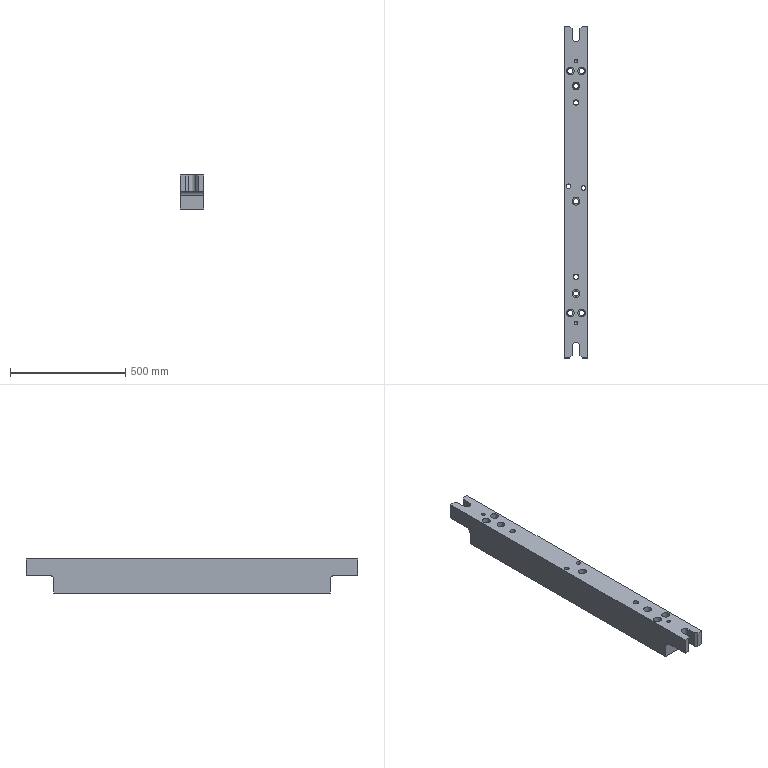Part | STEP file | lll_id2302_x_t | 1 solid | 57 faces | box 100 x 1440 x 147.5 mm | volume 18089858 mm3 | plane 29 | cylinder 26 | cone 2 | commonest cylinder face diameters 23.009 x7 34.008 x7 20 x4 14.506 x2 24 x2 34 x2
STEP:
#1=CARTESIAN_POINT('',(345.5,24.75,222.5));
#2=VERTEX_POINT('',#1);
#3=CARTESIAN_POINT('',(335.5,24.75,222.5));
#4=DIRECTION('',(0.,0.,1.));
#5=DIRECTION('',(1.,0.,0.));
#6=AXIS2_PLACEMENT_3D('',#3,#4,#5);
#7=CIRCLE('',#6,10.);
#8=EDGE_CURVE('',#2,#2,#7,.T.);
#9=ORIENTED_EDGE('',*,*,#8,.T.);
#10=EDGE_LOOP('',(#9));
#11=FACE_BOUND('',#10,.T.);
#12=CARTESIAN_POINT('',(317.435,-600.,222.5));
#13=VERTEX_POINT('',#12);
#14=CARTESIAN_POINT('',(317.435,600.,222.5));
#15=VERTEX_POINT('',#14);
#16=CARTESIAN_POINT('',(317.435,-1.,222.5));
#17=DIRECTION('',(0.,1.,0.));
#18=VECTOR('',#17,1.);
#19=LINE('',#16,#18);
#20=EDGE_CURVE('',#13,#15,#19,.T.);
#21=ORIENTED_EDGE('',*,*,#20,.T.);
#22=CARTESIAN_POINT('',(417.435,600.,222.5));
#23=VERTEX_POINT('',#22);
#24=CARTESIAN_POINT('',(-1848.88,600.,222.5));
#25=DIRECTION('',(1.,0.,0.));
#26=VECTOR('',#25,1.);
#27=LINE('',#24,#26);
#28=EDGE_CURVE('',#15,#23,#27,.T.);
#29=ORIENTED_EDGE('',*,*,#28,.T.);
#30=CARTESIAN_POINT('',(417.435,-600.,222.5));
#31=VERTEX_POINT('',#30);
#32=CARTESIAN_POINT('',(417.435,-1.,222.5));
#33=DIRECTION('',(0.,1.,0.));
#34=VECTOR('',#33,1.);
#35=LINE('',#32,#34);
#36=EDGE_CURVE('',#31,#23,#35,.T.);
#37=ORIENTED_EDGE('',*,*,#36,.F.);
#38=CARTESIAN_POINT('',(-1848.88,-600.,222.5));
#39=DIRECTION('',(-1.,0.,0.));
#40=VECTOR('',#39,1.);
#41=LINE('',#38,#40);
#42=EDGE_CURVE('',#31,#13,#41,.T.);
#43=ORIENTED_EDGE('',*,*,#42,.T.);
#44=EDGE_LOOP('',(#21,#29,#37,#43));
#45=FACE_BOUND('',#44,.T.);
#46=CARTESIAN_POINT('',(380.931,-525.,222.5));
#47=VERTEX_POINT('',#46);
#48=CARTESIAN_POINT('',(392.435,-525.,222.5));
#49=DIRECTION('',(0.,0.,-1.));
#50=DIRECTION('',(-1.,0.,0.));
#51=AXIS2_PLACEMENT_3D('',#48,#49,#50);
#52=CIRCLE('',#51,11.505);
#53=EDGE_CURVE('',#47,#47,#52,.T.);
#54=ORIENTED_EDGE('',*,*,#53,.F.);
#55=EDGE_LOOP('',(#54));
#56=FACE_BOUND('',#55,.T.);
#57=CARTESIAN_POINT('',(357.435,-368.,222.5));
#58=VERTEX_POINT('',#57);
#59=CARTESIAN_POINT('',(367.435,-368.,222.5));
#60=DIRECTION('',(0.,0.,-1.));
#61=DIRECTION('',(-1.,0.,0.));
#62=AXIS2_PLACEMENT_3D('',#59,#60,#61);
#63=CIRCLE('',#62,10.);
#64=EDGE_CURVE('',#58,#58,#63,.T.);
#65=ORIENTED_EDGE('',*,*,#64,.F.);
#66=EDGE_LOOP('',(#65));
#67=FACE_BOUND('',#66,.T.);
#68=CARTESIAN_POINT('',(355.931,-440.,222.5));
#69=VERTEX_POINT('',#68);
#70=CARTESIAN_POINT('',(367.435,-440.,222.5));
#71=DIRECTION('',(0.,0.,-1.));
#72=DIRECTION('',(-1.,0.,0.));
#73=AXIS2_PLACEMENT_3D('',#70,#71,#72);
#74=CIRCLE('',#73,11.505);
#75=EDGE_CURVE('',#69,#69,#74,.T.);
#76=ORIENTED_EDGE('',*,*,#75,.F.);
#77=EDGE_LOOP('',(#76));
#78=FACE_BOUND('',#77,.T.);
#79=CARTESIAN_POINT('',(330.931,-525.,222.5));
#80=VERTEX_POINT('',#79);
#81=CARTESIAN_POINT('',(342.435,-525.,222.5));
#82=DIRECTION('',(0.,0.,-1.));
#83=DIRECTION('',(-1.,0.,0.));
#84=AXIS2_PLACEMENT_3D('',#81,#82,#83);
#85=CIRCLE('',#84,11.505);
#86=EDGE_CURVE('',#80,#80,#85,.T.);
#87=ORIENTED_EDGE('',*,*,#86,.F.);
#88=EDGE_LOOP('',(#87));
#89=FACE_BOUND('',#88,.T.);
#90=CARTESIAN_POINT('',(353.94,525.,222.5));
#91=VERTEX_POINT('',#90);
#92=CARTESIAN_POINT('',(342.435,525.,222.5));
#93=DIRECTION('',(0.,0.,-1.));
#94=DIRECTION('',(1.,0.,0.));
#95=AXIS2_PLACEMENT_3D('',#92,#93,#94);
#96=CIRCLE('',#95,11.505);
#97=EDGE_CURVE('',#91,#91,#96,.T.);
#98=ORIENTED_EDGE('',*,*,#97,.F.);
#99=EDGE_LOOP('',(#98));
#100=FACE_BOUND('',#99,.T.);
#101=CARTESIAN_POINT('',(403.94,525.,222.5));
#102=VERTEX_POINT('',#101);
#103=CARTESIAN_POINT('',(392.435,525.,222.5));
#104=DIRECTION('',(0.,0.,-1.));
#105=DIRECTION('',(1.,0.,0.));
#106=AXIS2_PLACEMENT_3D('',#103,#104,#105);
#107=CIRCLE('',#106,11.505);
#108=EDGE_CURVE('',#102,#102,#107,.T.);
#109=ORIENTED_EDGE('',*,*,#108,.F.);
#110=EDGE_LOOP('',(#109));
#111=FACE_BOUND('',#110,.T.);
#112=CARTESIAN_POINT('',(378.94,460.,222.5));
#113=VERTEX_POINT('',#112);
#114=CARTESIAN_POINT('',(367.435,460.,222.5));
#115=DIRECTION('',(0.,0.,-1.));
#116=DIRECTION('',(1.,0.,0.));
#117=AXIS2_PLACEMENT_3D('',#114,#115,#116);
#118=CIRCLE('',#117,11.505);
#119=EDGE_CURVE('',#113,#113,#118,.T.);
#120=ORIENTED_EDGE('',*,*,#119,.F.);
#121=EDGE_LOOP('',(#120));
#122=FACE_BOUND('',#121,.T.);
#123=CARTESIAN_POINT('',(378.94,-40.,222.5));
#124=VERTEX_POINT('',#123);
#125=CARTESIAN_POINT('',(367.435,-40.,222.5));
#126=DIRECTION('',(0.,0.,-1.));
#127=DIRECTION('',(1.,0.,0.));
#128=AXIS2_PLACEMENT_3D('',#125,#126,#127);
#129=CIRCLE('',#128,11.505);
#130=EDGE_CURVE('',#124,#124,#129,.T.);
#131=ORIENTED_EDGE('',*,*,#130,.F.);
#132=EDGE_LOOP('',(#131));
#133=FACE_BOUND('',#132,.T.);
#134=CARTESIAN_POINT('',(377.435,388.,222.5));
#135=VERTEX_POINT('',#134);
#136=CARTESIAN_POINT('',(367.435,388.,222.5));
#137=DIRECTION('',(0.,0.,1.));
#138=DIRECTION('',(1.,0.,0.));
#139=AXIS2_PLACEMENT_3D('',#136,#137,#138);
#140=CIRCLE('',#139,10.);
#141=EDGE_CURVE('',#135,#135,#140,.T.);
#142=ORIENTED_EDGE('',*,*,#141,.T.);
#143=EDGE_LOOP('',(#142));
#144=FACE_BOUND('',#143,.T.);
#145=CARTESIAN_POINT('',(410.5,17.75,222.5));
#146=VERTEX_POINT('',#145);
#147=CARTESIAN_POINT('',(400.5,17.75,222.5));
#148=DIRECTION('',(0.,0.,1.));
#149=DIRECTION('',(1.,0.,0.));
#150=AXIS2_PLACEMENT_3D('',#147,#148,#149);
#151=CIRCLE('',#150,10.);
#152=EDGE_CURVE('',#146,#146,#151,.T.);
#153=ORIENTED_EDGE('',*,*,#152,.T.);
#154=EDGE_LOOP('',(#153));
#155=FACE_BOUND('',#154,.T.);
#156=CARTESIAN_POINT('',(-1848.88,-1.,222.5));
#157=DIRECTION('',(0.,0.,-1.));
#158=DIRECTION('',(1.,0.,0.));
#159=AXIS2_PLACEMENT_3D('',#156,#157,#158);
#160=PLANE('',#159);
#161=ADVANCED_FACE('',(#11,#45,#56,#67,#78,#89,#100,#111,#122,#133,#144,#155),#160,.T.);
#162=CARTESIAN_POINT('',(390.5,17.75,370.));
#163=VERTEX_POINT('',#162);
#164=CARTESIAN_POINT('',(400.5,17.75,370.));
#165=DIRECTION('',(0.,0.,-1.));
#166=DIRECTION('',(-1.,0.,0.));
#167=AXIS2_PLACEMENT_3D('',#164,#165,#166);
#168=CIRCLE('',#167,10.);
#169=EDGE_CURVE('',#163,#163,#168,.T.);
#170=ORIENTED_EDGE('',*,*,#169,.T.);
#171=EDGE_LOOP('',(#170));
#172=FACE_BOUND('',#171,.T.);
#173=CARTESIAN_POINT('',(325.5,24.75,370.));
#174=VERTEX_POINT('',#173);
#175=CARTESIAN_POINT('',(335.5,24.75,370.));
#176=DIRECTION('',(0.,0.,-1.));
#177=DIRECTION('',(-1.,0.,0.));
#178=AXIS2_PLACEMENT_3D('',#175,#176,#177);
#179=CIRCLE('',#178,10.);
#180=EDGE_CURVE('',#174,#174,#179,.T.);
#181=ORIENTED_EDGE('',*,*,#180,.T.);
#182=EDGE_LOOP('',(#181));
#183=FACE_BOUND('',#182,.T.);
#184=CARTESIAN_POINT('',(317.435,-720.,370.));
#185=VERTEX_POINT('',#184);
#186=CARTESIAN_POINT('',(317.435,720.,370.));
#187=VERTEX_POINT('',#186);
#188=CARTESIAN_POINT('',(317.435,-1.,370.));
#189=DIRECTION('',(0.,1.,0.));
#190=VECTOR('',#189,1.);
#191=LINE('',#188,#190);
#192=EDGE_CURVE('',#185,#187,#191,.T.);
#193=ORIENTED_EDGE('',*,*,#192,.F.);
#194=CARTESIAN_POINT('',(340.435,-720.,370.));
#195=VERTEX_POINT('',#194);
#196=CARTESIAN_POINT('',(-1848.88,-720.,370.));
#197=DIRECTION('',(-1.,0.,0.));
#198=VECTOR('',#197,1.);
#199=LINE('',#196,#198);
#200=EDGE_CURVE('',#195,#185,#199,.T.);
#201=ORIENTED_EDGE('',*,*,#200,.F.);
#202=CARTESIAN_POINT('',(350.435,-710.,370.));
#203=VERTEX_POINT('',#202);
#204=CARTESIAN_POINT('',(350.435,-710.,370.));
#205=DIRECTION('',(0.7071,0.7071,0.));
#206=VECTOR('',#205,1.);
#207=LINE('',#204,#206);
#208=EDGE_CURVE('',#195,#203,#207,.T.);
#209=ORIENTED_EDGE('',*,*,#208,.T.);
#210=CARTESIAN_POINT('',(350.435,-670.,370.));
#211=VERTEX_POINT('',#210);
#212=CARTESIAN_POINT('',(350.435,120.,370.));
#213=DIRECTION('',(0.,-1.,0.));
#214=VECTOR('',#213,1.);
#215=LINE('',#212,#214);
#216=EDGE_CURVE('',#211,#203,#215,.T.);
#217=ORIENTED_EDGE('',*,*,#216,.F.);
#218=CARTESIAN_POINT('',(384.435,-670.,370.));
#219=VERTEX_POINT('',#218);
#220=CARTESIAN_POINT('',(367.435,-670.,370.));
#221=DIRECTION('',(0.,0.,1.));
#222=DIRECTION('',(1.,0.,0.));
#223=AXIS2_PLACEMENT_3D('',#220,#221,#222);
#224=CIRCLE('',#223,17.);
#225=EDGE_CURVE('',#219,#211,#224,.T.);
#226=ORIENTED_EDGE('',*,*,#225,.F.);
#227=CARTESIAN_POINT('',(384.435,-710.,370.));
#228=VERTEX_POINT('',#227);
#229=CARTESIAN_POINT('',(384.435,120.,370.));
#230=DIRECTION('',(0.,1.,0.));
#231=VECTOR('',#230,1.);
#232=LINE('',#229,#231);
#233=EDGE_CURVE('',#228,#219,#232,.T.);
#234=ORIENTED_EDGE('',*,*,#233,.F.);
#235=CARTESIAN_POINT('',(394.435,-720.,370.));
#236=VERTEX_POINT('',#235);
#237=CARTESIAN_POINT('',(384.435,-710.,370.));
#238=DIRECTION('',(0.7071,-0.7071,0.));
#239=VECTOR('',#238,1.);
#240=LINE('',#237,#239);
#241=EDGE_CURVE('',#228,#236,#240,.T.);
#242=ORIENTED_EDGE('',*,*,#241,.T.);
#243=CARTESIAN_POINT('',(417.435,-720.,370.));
#244=VERTEX_POINT('',#243);
#245=CARTESIAN_POINT('',(-1848.88,-720.,370.));
#246=DIRECTION('',(-1.,0.,0.));
#247=VECTOR('',#246,1.);
#248=LINE('',#245,#247);
#249=EDGE_CURVE('',#244,#236,#248,.T.);
#250=ORIENTED_EDGE('',*,*,#249,.F.);
#251=CARTESIAN_POINT('',(417.435,720.,370.));
#252=VERTEX_POINT('',#251);
#253=CARTESIAN_POINT('',(417.435,0.,370.));
#254=DIRECTION('',(0.,-1.,0.));
#255=VECTOR('',#254,1.);
#256=LINE('',#253,#255);
#257=EDGE_CURVE('',#252,#244,#256,.T.);
#258=ORIENTED_EDGE('',*,*,#257,.F.);
#259=CARTESIAN_POINT('',(394.435,720.,370.));
#260=VERTEX_POINT('',#259);
#261=CARTESIAN_POINT('',(-1848.88,720.,370.));
#262=DIRECTION('',(1.,0.,0.));
#263=VECTOR('',#262,1.);
#264=LINE('',#261,#263);
#265=EDGE_CURVE('',#260,#252,#264,.T.);
#266=ORIENTED_EDGE('',*,*,#265,.F.);
#267=CARTESIAN_POINT('',(384.435,710.,370.));
#268=VERTEX_POINT('',#267);
#269=CARTESIAN_POINT('',(350.935,676.5,370.));
#270=DIRECTION('',(0.7071,0.7071,0.));
#271=VECTOR('',#270,1.);
#272=LINE('',#269,#271);
#273=EDGE_CURVE('',#268,#260,#272,.T.);
#274=ORIENTED_EDGE('',*,*,#273,.F.);
#275=CARTESIAN_POINT('',(384.435,670.,370.));
#276=VERTEX_POINT('',#275);
#277=CARTESIAN_POINT('',(384.435,-120.,370.));
#278=DIRECTION('',(0.,-1.,0.));
#279=VECTOR('',#278,1.);
#280=LINE('',#277,#279);
#281=EDGE_CURVE('',#268,#276,#280,.T.);
#282=ORIENTED_EDGE('',*,*,#281,.T.);
#283=CARTESIAN_POINT('',(350.435,670.,370.));
#284=VERTEX_POINT('',#283);
#285=CARTESIAN_POINT('',(367.435,670.,370.));
#286=DIRECTION('',(0.,0.,-1.));
#287=DIRECTION('',(1.,0.,0.));
#288=AXIS2_PLACEMENT_3D('',#285,#286,#287);
#289=CIRCLE('',#288,17.);
#290=EDGE_CURVE('',#276,#284,#289,.T.);
#291=ORIENTED_EDGE('',*,*,#290,.T.);
#292=CARTESIAN_POINT('',(350.435,710.,370.));
#293=VERTEX_POINT('',#292);
#294=CARTESIAN_POINT('',(350.435,-120.,370.));
#295=DIRECTION('',(0.,1.,0.));
#296=VECTOR('',#295,1.);
#297=LINE('',#294,#296);
#298=EDGE_CURVE('',#284,#293,#297,.T.);
#299=ORIENTED_EDGE('',*,*,#298,.T.);
#300=CARTESIAN_POINT('',(340.435,720.,370.));
#301=VERTEX_POINT('',#300);
#302=CARTESIAN_POINT('',(1043.935,16.5,370.));
#303=DIRECTION('',(0.7071,-0.7071,0.));
#304=VECTOR('',#303,1.);
#305=LINE('',#302,#304);
#306=EDGE_CURVE('',#301,#293,#305,.T.);
#307=ORIENTED_EDGE('',*,*,#306,.F.);
#308=CARTESIAN_POINT('',(-1848.88,720.,370.));
#309=DIRECTION('',(1.,0.,0.));
#310=VECTOR('',#309,1.);
#311=LINE('',#308,#310);
#312=EDGE_CURVE('',#187,#301,#311,.T.);
#313=ORIENTED_EDGE('',*,*,#312,.F.);
#314=EDGE_LOOP('',(#193,#201,#209,#217,#226,#234,#242,#250,#258,#266,#274,#282,#291,#299,#307,#313));
#315=FACE_BOUND('',#314,.T.);
#316=CARTESIAN_POINT('',(374.688,-568.,370.));
#317=VERTEX_POINT('',#316);
#318=CARTESIAN_POINT('',(367.435,-568.,370.));
#319=DIRECTION('',(0.,0.,-1.));
#320=DIRECTION('',(1.,0.,0.));
#321=AXIS2_PLACEMENT_3D('',#318,#319,#320);
#322=CIRCLE('',#321,7.253);
#323=EDGE_CURVE('',#317,#317,#322,.T.);
#324=ORIENTED_EDGE('',*,*,#323,.T.);
#325=EDGE_LOOP('',(#324));
#326=FACE_BOUND('',#325,.T.);
#327=CARTESIAN_POINT('',(374.688,568.,370.));
#328=VERTEX_POINT('',#327);
#329=CARTESIAN_POINT('',(367.435,568.,370.));
#330=DIRECTION('',(0.,0.,1.));
#331=DIRECTION('',(1.,0.,0.));
#332=AXIS2_PLACEMENT_3D('',#329,#330,#331);
#333=CIRCLE('',#332,7.253);
#334=EDGE_CURVE('',#328,#328,#333,.T.);
#335=ORIENTED_EDGE('',*,*,#334,.F.);
#336=EDGE_LOOP('',(#335));
#337=FACE_BOUND('',#336,.T.);
#338=CARTESIAN_POINT('',(375.431,-525.,370.));
#339=VERTEX_POINT('',#338);
#340=CARTESIAN_POINT('',(392.435,-525.,370.));
#341=DIRECTION('',(0.,0.,-1.));
#342=DIRECTION('',(-1.,0.,0.));
#343=AXIS2_PLACEMENT_3D('',#340,#341,#342);
#344=CIRCLE('',#343,17.004);
#345=EDGE_CURVE('',#339,#339,#344,.T.);
#346=ORIENTED_EDGE('',*,*,#345,.T.);
#347=EDGE_LOOP('',(#346));
#348=FACE_BOUND('',#347,.T.);
#349=CARTESIAN_POINT('',(355.435,-368.,370.));
#350=VERTEX_POINT('',#349);
#351=CARTESIAN_POINT('',(367.435,-368.,370.));
#352=DIRECTION('',(0.,0.,-1.));
#353=DIRECTION('',(-1.,0.,0.));
#354=AXIS2_PLACEMENT_3D('',#351,#352,#353);
#355=CIRCLE('',#354,12.);
#356=EDGE_CURVE('',#350,#350,#355,.T.);
#357=ORIENTED_EDGE('',*,*,#356,.T.);
#358=EDGE_LOOP('',(#357));
#359=FACE_BOUND('',#358,.T.);
#360=CARTESIAN_POINT('',(350.431,-440.,370.));
#361=VERTEX_POINT('',#360);
#362=CARTESIAN_POINT('',(367.435,-440.,370.));
#363=DIRECTION('',(0.,0.,-1.));
#364=DIRECTION('',(-1.,0.,0.));
#365=AXIS2_PLACEMENT_3D('',#362,#363,#364);
#366=CIRCLE('',#365,17.004);
#367=EDGE_CURVE('',#361,#361,#366,.T.);
#368=ORIENTED_EDGE('',*,*,#367,.T.);
#369=EDGE_LOOP('',(#368));
#370=FACE_BOUND('',#369,.T.);
#371=CARTESIAN_POINT('',(325.431,-525.,370.));
#372=VERTEX_POINT('',#371);
#373=CARTESIAN_POINT('',(342.435,-525.,370.));
#374=DIRECTION('',(0.,0.,-1.));
#375=DIRECTION('',(-1.,0.,0.));
#376=AXIS2_PLACEMENT_3D('',#373,#374,#375);
#377=CIRCLE('',#376,17.004);
#378=EDGE_CURVE('',#372,#372,#377,.T.);
#379=ORIENTED_EDGE('',*,*,#378,.T.);
#380=EDGE_LOOP('',(#379));
#381=FACE_BOUND('',#380,.T.);
#382=CARTESIAN_POINT('',(375.431,525.,370.));
#383=VERTEX_POINT('',#382);
#384=CARTESIAN_POINT('',(392.435,525.,370.));
#385=DIRECTION('',(0.,0.,1.));
#386=DIRECTION('',(-1.,0.,0.));
#387=AXIS2_PLACEMENT_3D('',#384,#385,#386);
#388=CIRCLE('',#387,17.004);
#389=EDGE_CURVE('',#383,#383,#388,.T.);
#390=ORIENTED_EDGE('',*,*,#389,.F.);
#391=EDGE_LOOP('',(#390));
#392=FACE_BOUND('',#391,.T.);
#393=CARTESIAN_POINT('',(359.439,525.,370.));
#394=VERTEX_POINT('',#393);
#395=CARTESIAN_POINT('',(342.435,525.,370.));
#396=DIRECTION('',(0.,0.,-1.));
#397=DIRECTION('',(1.,0.,0.));
#398=AXIS2_PLACEMENT_3D('',#395,#396,#397);
#399=CIRCLE('',#398,17.004);
#400=EDGE_CURVE('',#394,#394,#399,.T.);
#401=ORIENTED_EDGE('',*,*,#400,.T.);
#402=EDGE_LOOP('',(#401));
#403=FACE_BOUND('',#402,.T.);
#404=CARTESIAN_POINT('',(384.439,460.,370.));
#405=VERTEX_POINT('',#404);
#406=CARTESIAN_POINT('',(367.435,460.,370.));
#407=DIRECTION('',(0.,0.,-1.));
#408=DIRECTION('',(1.,0.,0.));
#409=AXIS2_PLACEMENT_3D('',#406,#407,#408);
#410=CIRCLE('',#409,17.004);
#411=EDGE_CURVE('',#405,#405,#410,.T.);
#412=ORIENTED_EDGE('',*,*,#411,.T.);
#413=EDGE_LOOP('',(#412));
#414=FACE_BOUND('',#413,.T.);
#415=CARTESIAN_POINT('',(384.439,-40.,370.));
#416=VERTEX_POINT('',#415);
#417=CARTESIAN_POINT('',(367.435,-40.,370.));
#418=DIRECTION('',(0.,0.,-1.));
#419=DIRECTION('',(1.,0.,0.));
#420=AXIS2_PLACEMENT_3D('',#417,#418,#419);
#421=CIRCLE('',#420,17.004);
#422=EDGE_CURVE('',#416,#416,#421,.T.);
#423=ORIENTED_EDGE('',*,*,#422,.T.);
#424=EDGE_LOOP('',(#423));
#425=FACE_BOUND('',#424,.T.);
#426=CARTESIAN_POINT('',(355.435,388.,370.));
#427=VERTEX_POINT('',#426);
#428=CARTESIAN_POINT('',(367.435,388.,370.));
#429=DIRECTION('',(0.,0.,-1.));
#430=DIRECTION('',(-1.,0.,0.));
#431=AXIS2_PLACEMENT_3D('',#428,#429,#430);
#432=CIRCLE('',#431,12.);
#433=EDGE_CURVE('',#427,#427,#432,.T.);
#434=ORIENTED_EDGE('',*,*,#433,.T.);
#435=EDGE_LOOP('',(#434));
#436=FACE_BOUND('',#435,.T.);
#437=CARTESIAN_POINT('',(-1848.88,-1.,370.));
#438=DIRECTION('',(0.,0.,-1.));
#439=DIRECTION('',(1.,0.,0.));
#440=AXIS2_PLACEMENT_3D('',#437,#438,#439);
#441=PLANE('',#440);
#442=ADVANCED_FACE('',(#172,#183,#315,#326,#337,#348,#359,#370,#381,#392,#403,#414,#425,#436),#441,.F.);
#443=CARTESIAN_POINT('',(330.931,-525.,272.5));
#444=VERTEX_POINT('',#443);
#445=CARTESIAN_POINT('',(342.435,-525.,272.5));
#446=DIRECTION('',(0.,0.,-1.));
#447=DIRECTION('',(-1.,0.,0.));
#448=AXIS2_PLACEMENT_3D('',#445,#446,#447);
#449=CIRCLE('',#448,11.505);
#450=EDGE_CURVE('',#444,#444,#449,.T.);
#451=ORIENTED_EDGE('',*,*,#450,.T.);
#452=EDGE_LOOP('',(#451));
#453=FACE_BOUND('',#452,.T.);
#454=CARTESIAN_POINT('',(359.439,-525.,272.5));
#455=VERTEX_POINT('',#454);
#456=CARTESIAN_POINT('',(342.435,-525.,272.5));
#457=DIRECTION('',(0.,0.,-1.));
#458=DIRECTION('',(1.,0.,0.));
#459=AXIS2_PLACEMENT_3D('',#456,#457,#458);
#460=CIRCLE('',#459,17.004);
#461=EDGE_CURVE('',#455,#455,#460,.T.);
#462=ORIENTED_EDGE('',*,*,#461,.F.);
#463=EDGE_LOOP('',(#462));
#464=FACE_BOUND('',#463,.T.);
#465=CARTESIAN_POINT('',(342.435,-545.,272.5));
#466=DIRECTION('',(0.,0.,-1.));
#467=DIRECTION('',(-1.,0.,0.));
#468=AXIS2_PLACEMENT_3D('',#465,#466,#467);
#469=PLANE('',#468);
#470=ADVANCED_FACE('',(#453,#464),#469,.F.);
#471=ORIENTED_EDGE('',*,*,#461,.T.);
#472=EDGE_LOOP('',(#471));
#473=FACE_BOUND('',#472,.T.);
#474=ORIENTED_EDGE('',*,*,#378,.F.);
#475=EDGE_LOOP('',(#474));
#476=FACE_BOUND('',#475,.T.);
#477=CARTESIAN_POINT('',(342.435,-525.,370.));
#478=DIRECTION('',(0.,0.,-1.));
#479=DIRECTION('',(1.,0.,0.));
#480=AXIS2_PLACEMENT_3D('',#477,#478,#479);
#481=CYLINDRICAL_SURFACE('',#480,17.004);
#482=ADVANCED_FACE('',(#473,#476),#481,.F.);
#483=ORIENTED_EDGE('',*,*,#86,.T.);
#484=EDGE_LOOP('',(#483));
#485=FACE_BOUND('',#484,.T.);
#486=ORIENTED_EDGE('',*,*,#450,.F.);
#487=EDGE_LOOP('',(#486));
#488=FACE_BOUND('',#487,.T.);
#489=CARTESIAN_POINT('',(342.435,-525.,422.));
#490=DIRECTION('',(0.,0.,-1.));
#491=DIRECTION('',(1.,0.,0.));
#492=AXIS2_PLACEMENT_3D('',#489,#490,#491);
#493=CYLINDRICAL_SURFACE('',#492,11.505);
#494=ADVANCED_FACE('',(#485,#488),#493,.F.);
#495=CARTESIAN_POINT('',(355.435,388.,270.));
#496=VERTEX_POINT('',#495);
#497=CARTESIAN_POINT('',(367.435,388.,270.));
#498=DIRECTION('',(0.,0.,1.));
#499=DIRECTION('',(-1.,0.,0.));
#500=AXIS2_PLACEMENT_3D('',#497,#498,#499);
#501=CIRCLE('',#500,12.);
#502=EDGE_CURVE('',#496,#496,#501,.T.);
#503=ORIENTED_EDGE('',*,*,#502,.T.);
#504=EDGE_LOOP('',(#503));
#505=FACE_BOUND('',#504,.T.);
#506=CARTESIAN_POINT('',(377.435,388.,270.));
#507=VERTEX_POINT('',#506);
#508=CARTESIAN_POINT('',(367.435,388.,270.));
#509=DIRECTION('',(0.,0.,-1.));
#510=DIRECTION('',(1.,0.,0.));
#511=AXIS2_PLACEMENT_3D('',#508,#509,#510);
#512=CIRCLE('',#511,10.);
#513=EDGE_CURVE('',#507,#507,#512,.T.);
#514=ORIENTED_EDGE('',*,*,#513,.T.);
#515=EDGE_LOOP('',(#514));
#516=FACE_BOUND('',#515,.T.);
#517=CARTESIAN_POINT('',(367.435,388.,270.));
#518=DIRECTION('',(0.,0.,-1.));
#519=DIRECTION('',(1.,0.,0.));
#520=AXIS2_PLACEMENT_3D('',#517,#518,#519);
#521=PLANE('',#520);
#522=ADVANCED_FACE('',(#505,#516),#521,.F.);
#523=CARTESIAN_POINT('',(355.931,-40.,272.5));
#524=VERTEX_POINT('',#523);
#525=CARTESIAN_POINT('',(367.435,-40.,272.5));
#526=DIRECTION('',(0.,0.,-1.));
#527=DIRECTION('',(-1.,0.,0.));
#528=AXIS2_PLACEMENT_3D('',#525,#526,#527);
#529=CIRCLE('',#528,11.505);
#530=EDGE_CURVE('',#524,#524,#529,.T.);
#531=ORIENTED_EDGE('',*,*,#530,.T.);
#532=EDGE_LOOP('',(#531));
#533=FACE_BOUND('',#532,.T.);
#534=CARTESIAN_POINT('',(384.439,-40.,272.5));
#535=VERTEX_POINT('',#534);
#536=CARTESIAN_POINT('',(367.435,-40.,272.5));
#537=DIRECTION('',(0.,0.,-1.));
#538=DIRECTION('',(1.,0.,0.));
#539=AXIS2_PLACEMENT_3D('',#536,#537,#538);
#540=CIRCLE('',#539,17.004);
#541=EDGE_CURVE('',#535,#535,#540,.T.);
#542=ORIENTED_EDGE('',*,*,#541,.F.);
#543=EDGE_LOOP('',(#542));
#544=FACE_BOUND('',#543,.T.);
#545=CARTESIAN_POINT('',(367.435,0.,272.5));
#546=DIRECTION('',(0.,0.,-1.));
#547=DIRECTION('',(-1.,0.,0.));
#548=AXIS2_PLACEMENT_3D('',#545,#546,#547);
#549=PLANE('',#548);
#550=ADVANCED_FACE('',(#533,#544),#549,.F.);
#551=CARTESIAN_POINT('',(355.931,460.,272.5));
#552=VERTEX_POINT('',#551);
#553=CARTESIAN_POINT('',(367.435,460.,272.5));
#554=DIRECTION('',(0.,0.,-1.));
#555=DIRECTION('',(-1.,0.,0.));
#556=AXIS2_PLACEMENT_3D('',#553,#554,#555);
#557=CIRCLE('',#556,11.505);
#558=EDGE_CURVE('',#552,#552,#557,.T.);
#559=ORIENTED_EDGE('',*,*,#558,.T.);
#560=EDGE_LOOP('',(#559));
#561=FACE_BOUND('',#560,.T.);
#562=CARTESIAN_POINT('',(384.439,460.,272.5));
#563=VERTEX_POINT('',#562);
#564=CARTESIAN_POINT('',(367.435,460.,272.5));
#565=DIRECTION('',(0.,0.,-1.));
#566=DIRECTION('',(1.,0.,0.));
#567=AXIS2_PLACEMENT_3D('',#564,#565,#566);
#568=CIRCLE('',#567,17.004);
#569=EDGE_CURVE('',#563,#563,#568,.T.);
#570=ORIENTED_EDGE('',*,*,#569,.F.);
#571=EDGE_LOOP('',(#570));
#572=FACE_BOUND('',#571,.T.);
#573=CARTESIAN_POINT('',(367.435,465.,272.5));
#574=DIRECTION('',(0.,0.,-1.));
#575=DIRECTION('',(-1.,0.,0.));
#576=AXIS2_PLACEMENT_3D('',#573,#574,#575);
#577=PLANE('',#576);
#578=ADVANCED_FACE('',(#561,#572),#577,.F.);
#579=CARTESIAN_POINT('',(330.931,525.,272.5));
#580=VERTEX_POINT('',#579);
#581=CARTESIAN_POINT('',(342.435,525.,272.5));
#582=DIRECTION('',(0.,0.,-1.));
#583=DIRECTION('',(-1.,0.,0.));
#584=AXIS2_PLACEMENT_3D('',#581,#582,#583);
#585=CIRCLE('',#584,11.505);
#586=EDGE_CURVE('',#580,#580,#585,.T.);
#587=ORIENTED_EDGE('',*,*,#586,.T.);
#588=EDGE_LOOP('',(#587));
#589=FACE_BOUND('',#588,.T.);
#590=CARTESIAN_POINT('',(359.439,525.,272.5));
#591=VERTEX_POINT('',#590);
#592=CARTESIAN_POINT('',(342.435,525.,272.5));
#593=DIRECTION('',(0.,0.,-1.));
#594=DIRECTION('',(1.,0.,0.));
#595=AXIS2_PLACEMENT_3D('',#592,#593,#594);
#596=CIRCLE('',#595,17.004);
#597=EDGE_CURVE('',#591,#591,#596,.T.);
#598=ORIENTED_EDGE('',*,*,#597,.F.);
#599=EDGE_LOOP('',(#598));
#600=FACE_BOUND('',#599,.T.);
#601=CARTESIAN_POINT('',(342.435,545.,272.5));
#602=DIRECTION('',(0.,0.,-1.));
#603=DIRECTION('',(-1.,0.,0.));
#604=AXIS2_PLACEMENT_3D('',#601,#602,#603);
#605=PLANE('',#604);
#606=ADVANCED_FACE('',(#589,#600),#605,.F.);
#607=CARTESIAN_POINT('',(403.94,525.,272.5));
#608=VERTEX_POINT('',#607);
#609=CARTESIAN_POINT('',(392.435,525.,272.5));
#610=DIRECTION('',(0.,0.,1.));
#611=DIRECTION('',(1.,0.,0.));
#612=AXIS2_PLACEMENT_3D('',#609,#610,#611);
#613=CIRCLE('',#612,11.505);
#614=EDGE_CURVE('',#608,#608,#613,.T.);
#615=ORIENTED_EDGE('',*,*,#614,.F.);
#616=EDGE_LOOP('',(#615));
#617=FACE_BOUND('',#616,.T.);
#618=CARTESIAN_POINT('',(375.431,525.,272.5));
#619=VERTEX_POINT('',#618);
#620=CARTESIAN_POINT('',(392.435,525.,272.5));
#621=DIRECTION('',(0.,0.,1.));
#622=DIRECTION('',(-1.,0.,0.));
#623=AXIS2_PLACEMENT_3D('',#620,#621,#622);
#624=CIRCLE('',#623,17.004);
#625=EDGE_CURVE('',#619,#619,#624,.T.);
#626=ORIENTED_EDGE('',*,*,#625,.T.);
#627=EDGE_LOOP('',(#626));
#628=FACE_BOUND('',#627,.T.);
#629=CARTESIAN_POINT('',(392.435,545.,272.5));
#630=DIRECTION('',(0.,0.,-1.));
#631=DIRECTION('',(1.,0.,0.));
#632=AXIS2_PLACEMENT_3D('',#629,#630,#631);
#633=PLANE('',#632);
#634=ADVANCED_FACE('',(#617,#628),#633,.F.);
#635=CARTESIAN_POINT('',(417.435,-720.,300.));
#636=VERTEX_POINT('',#635);
#637=CARTESIAN_POINT('',(394.435,-720.,300.));
#638=VERTEX_POINT('',#637);
#639=CARTESIAN_POINT('',(367.435,-720.,300.));
#640=DIRECTION('',(-1.,0.,0.));
#641=VECTOR('',#640,1.);
#642=LINE('',#639,#641);
#643=EDGE_CURVE('',#636,#638,#642,.T.);
#644=ORIENTED_EDGE('',*,*,#643,.T.);
#645=CARTESIAN_POINT('',(384.435,-710.,300.));
#646=VERTEX_POINT('',#645);
#647=CARTESIAN_POINT('',(361.685,-687.25,300.));
#648=DIRECTION('',(-0.7071,0.7071,0.));
#649=VECTOR('',#648,1.);
#650=LINE('',#647,#649);
#651=EDGE_CURVE('',#638,#646,#650,.T.);
#652=ORIENTED_EDGE('',*,*,#651,.T.);
#653=CARTESIAN_POINT('',(384.435,-670.,300.));
#654=VERTEX_POINT('',#653);
#655=CARTESIAN_POINT('',(384.435,-661.5,300.));
#656=DIRECTION('',(0.,-1.,0.));
#657=VECTOR('',#656,1.);
#658=LINE('',#655,#657);
#659=EDGE_CURVE('',#654,#646,#658,.T.);
#660=ORIENTED_EDGE('',*,*,#659,.F.);
#661=CARTESIAN_POINT('',(350.435,-670.,300.));
#662=VERTEX_POINT('',#661);
#663=CARTESIAN_POINT('',(367.435,-670.,300.));
#664=DIRECTION('',(0.,0.,1.));
#665=DIRECTION('',(1.,0.,0.));
#666=AXIS2_PLACEMENT_3D('',#663,#664,#665);
#667=CIRCLE('',#666,17.);
#668=EDGE_CURVE('',#654,#662,#667,.T.);
#669=ORIENTED_EDGE('',*,*,#668,.T.);
#670=CARTESIAN_POINT('',(350.435,-710.,300.));
#671=VERTEX_POINT('',#670);
#672=CARTESIAN_POINT('',(350.435,-661.5,300.));
#673=DIRECTION('',(0.,1.,0.));
#674=VECTOR('',#673,1.);
#675=LINE('',#672,#674);
#676=EDGE_CURVE('',#671,#662,#675,.T.);
#677=ORIENTED_EDGE('',*,*,#676,.F.);
#678=CARTESIAN_POINT('',(340.435,-720.,300.));
#679=VERTEX_POINT('',#678);
#680=CARTESIAN_POINT('',(373.185,-687.25,300.));
#681=DIRECTION('',(-0.7071,-0.7071,0.));
#682=VECTOR('',#681,1.);
#683=LINE('',#680,#682);
#684=EDGE_CURVE('',#671,#679,#683,.T.);
#685=ORIENTED_EDGE('',*,*,#684,.T.);
#686=CARTESIAN_POINT('',(317.435,-720.,300.));
#687=VERTEX_POINT('',#686);
#688=CARTESIAN_POINT('',(367.435,-720.,300.));
#689=DIRECTION('',(-1.,0.,0.));
#690=VECTOR('',#689,1.);
#691=LINE('',#688,#690);
#692=EDGE_CURVE('',#679,#687,#691,.T.);
#693=ORIENTED_EDGE('',*,*,#692,.T.);
#694=CARTESIAN_POINT('',(317.435,-620.,300.));
#695=VERTEX_POINT('',#694);
#696=CARTESIAN_POINT('',(317.435,-681.5,300.));
#697=DIRECTION('',(0.,1.,0.));
#698=VECTOR('',#697,1.);
#699=LINE('',#696,#698);
#700=EDGE_CURVE('',#687,#695,#699,.T.);
#701=ORIENTED_EDGE('',*,*,#700,.T.);
#702=CARTESIAN_POINT('',(417.435,-620.,300.));
#703=VERTEX_POINT('',#702);
#704=CARTESIAN_POINT('',(407.435,-620.,300.));
#705=DIRECTION('',(1.,0.,0.));
#706=VECTOR('',#705,1.);
#707=LINE('',#704,#706);
#708=EDGE_CURVE('',#695,#703,#707,.T.);
#709=ORIENTED_EDGE('',*,*,#708,.T.);
#710=CARTESIAN_POINT('',(417.435,-681.5,300.));
#711=DIRECTION('',(0.,1.,0.));
#712=VECTOR('',#711,1.);
#713=LINE('',#710,#712);
#714=EDGE_CURVE('',#636,#703,#713,.T.);
#715=ORIENTED_EDGE('',*,*,#714,.F.);
#716=EDGE_LOOP('',(#644,#652,#660,#669,#677,#685,#693,#701,#709,#715));
#717=FACE_OUTER_BOUND('',#716,.T.);
#718=CARTESIAN_POINT('',(367.435,-681.5,300.));
#719=DIRECTION('',(0.,0.,-1.));
#720=DIRECTION('',(1.,0.,0.));
#721=AXIS2_PLACEMENT_3D('',#718,#719,#720);
#722=PLANE('',#721);
#723=ADVANCED_FACE('',(#717),#722,.T.);
#724=CARTESIAN_POINT('',(317.435,-600.,280.));
#725=VERTEX_POINT('',#724);
#726=CARTESIAN_POINT('',(317.435,-620.,280.));
#727=DIRECTION('',(1.,0.,0.));
#728=DIRECTION('',(0.,0.,-1.));
#729=AXIS2_PLACEMENT_3D('',#726,#727,#728);
#730=CIRCLE('',#729,20.);
#731=EDGE_CURVE('',#725,#695,#730,.T.);
#732=ORIENTED_EDGE('',*,*,#731,.F.);
#733=CARTESIAN_POINT('',(417.435,-600.,280.));
#734=VERTEX_POINT('',#733);
#735=CARTESIAN_POINT('',(327.435,-600.,280.));
#736=DIRECTION('',(-1.,0.,0.));
#737=VECTOR('',#736,1.);
#738=LINE('',#735,#737);
#739=EDGE_CURVE('',#734,#725,#738,.T.);
#740=ORIENTED_EDGE('',*,*,#739,.F.);
#741=CARTESIAN_POINT('',(417.435,-620.,280.));
#742=DIRECTION('',(-1.,0.,0.));
#743=DIRECTION('',(0.,0.,-1.));
#744=AXIS2_PLACEMENT_3D('',#741,#742,#743);
#745=CIRCLE('',#744,20.);
#746=EDGE_CURVE('',#703,#734,#745,.T.);
#747=ORIENTED_EDGE('',*,*,#746,.F.);
#748=ORIENTED_EDGE('',*,*,#708,.F.);
#749=EDGE_LOOP('',(#732,#740,#747,#748));
#750=FACE_OUTER_BOUND('',#749,.T.);
#751=CARTESIAN_POINT('',(367.435,-620.,280.));
#752=DIRECTION('',(-1.,0.,0.));
#753=DIRECTION('',(0.,0.,-1.));
#754=AXIS2_PLACEMENT_3D('',#751,#752,#753);
#755=CYLINDRICAL_SURFACE('',#754,20.);
#756=ADVANCED_FACE('',(#750),#755,.F.);
#757=CARTESIAN_POINT('',(417.435,600.,280.));
#758=VERTEX_POINT('',#757);
#759=CARTESIAN_POINT('',(417.435,620.,300.));
#760=VERTEX_POINT('',#759);
#761=CARTESIAN_POINT('',(417.435,620.,280.));
#762=DIRECTION('',(-1.,0.,0.));
#763=DIRECTION('',(0.,0.,-1.));
#764=AXIS2_PLACEMENT_3D('',#761,#762,#763);
#765=CIRCLE('',#764,20.);
#766=EDGE_CURVE('',#758,#760,#765,.T.);
#767=ORIENTED_EDGE('',*,*,#766,.F.);
#768=CARTESIAN_POINT('',(317.435,600.,280.));
#769=VERTEX_POINT('',#768);
#770=CARTESIAN_POINT('',(407.435,600.,280.));
#771=DIRECTION('',(1.,0.,0.));
#772=VECTOR('',#771,1.);
#773=LINE('',#770,#772);
#774=EDGE_CURVE('',#769,#758,#773,.T.);
#775=ORIENTED_EDGE('',*,*,#774,.F.);
#776=CARTESIAN_POINT('',(317.435,620.,300.));
#777=VERTEX_POINT('',#776);
#778=CARTESIAN_POINT('',(317.435,620.,280.));
#779=DIRECTION('',(1.,0.,0.));
#780=DIRECTION('',(0.,0.,-1.));
#781=AXIS2_PLACEMENT_3D('',#778,#779,#780);
#782=CIRCLE('',#781,20.);
#783=EDGE_CURVE('',#777,#769,#782,.T.);
#784=ORIENTED_EDGE('',*,*,#783,.F.);
#785=CARTESIAN_POINT('',(327.435,620.,300.));
#786=DIRECTION('',(-1.,0.,0.));
#787=VECTOR('',#786,1.);
#788=LINE('',#785,#787);
#789=EDGE_CURVE('',#760,#777,#788,.T.);
#790=ORIENTED_EDGE('',*,*,#789,.F.);
#791=EDGE_LOOP('',(#767,#775,#784,#790));
#792=FACE_OUTER_BOUND('',#791,.T.);
#793=CARTESIAN_POINT('',(367.435,620.,280.));
#794=DIRECTION('',(1.,0.,0.));
#795=DIRECTION('',(0.,0.,1.));
#796=AXIS2_PLACEMENT_3D('',#793,#794,#795);
#797=CYLINDRICAL_SURFACE('',#796,20.);
#798=ADVANCED_FACE('',(#792),#797,.F.);
#799=CARTESIAN_POINT('',(417.435,720.,300.));
#800=VERTEX_POINT('',#799);
#801=CARTESIAN_POINT('',(417.435,-641.5,300.));
#802=DIRECTION('',(0.,1.,0.));
#803=VECTOR('',#802,1.);
#804=LINE('',#801,#803);
#805=EDGE_CURVE('',#760,#800,#804,.T.);
#806=ORIENTED_EDGE('',*,*,#805,.F.);
#807=ORIENTED_EDGE('',*,*,#789,.T.);
#808=CARTESIAN_POINT('',(317.435,720.,300.));
#809=VERTEX_POINT('',#808);
#810=CARTESIAN_POINT('',(317.435,-641.5,300.));
#811=DIRECTION('',(0.,1.,0.));
#812=VECTOR('',#811,1.);
#813=LINE('',#810,#812);
#814=EDGE_CURVE('',#777,#809,#813,.T.);
#815=ORIENTED_EDGE('',*,*,#814,.T.);
#816=CARTESIAN_POINT('',(340.435,720.,300.));
#817=VERTEX_POINT('',#816);
#818=CARTESIAN_POINT('',(367.435,720.,300.));
#819=DIRECTION('',(1.,0.,0.));
#820=VECTOR('',#819,1.);
#821=LINE('',#818,#820);
#822=EDGE_CURVE('',#809,#817,#821,.T.);
#823=ORIENTED_EDGE('',*,*,#822,.T.);
#824=CARTESIAN_POINT('',(350.435,710.,300.));
#825=VERTEX_POINT('',#824);
#826=CARTESIAN_POINT('',(340.435,720.,300.));
#827=DIRECTION('',(0.7071,-0.7071,0.));
#828=VECTOR('',#827,1.);
#829=LINE('',#826,#828);
#830=EDGE_CURVE('',#817,#825,#829,.T.);
#831=ORIENTED_EDGE('',*,*,#830,.T.);
#832=CARTESIAN_POINT('',(350.435,670.,300.));
#833=VERTEX_POINT('',#832);
#834=CARTESIAN_POINT('',(350.435,-641.5,300.));
#835=DIRECTION('',(0.,-1.,0.));
#836=VECTOR('',#835,1.);
#837=LINE('',#834,#836);
#838=EDGE_CURVE('',#825,#833,#837,.T.);
#839=ORIENTED_EDGE('',*,*,#838,.T.);
#840=CARTESIAN_POINT('',(384.435,670.,300.));
#841=VERTEX_POINT('',#840);
#842=CARTESIAN_POINT('',(367.435,670.,300.));
#843=DIRECTION('',(0.,0.,-1.));
#844=DIRECTION('',(-1.,0.,0.));
#845=AXIS2_PLACEMENT_3D('',#842,#843,#844);
#846=CIRCLE('',#845,17.);
#847=EDGE_CURVE('',#841,#833,#846,.T.);
#848=ORIENTED_EDGE('',*,*,#847,.F.);
#849=CARTESIAN_POINT('',(384.435,710.,300.));
#850=VERTEX_POINT('',#849);
#851=CARTESIAN_POINT('',(384.435,-641.5,300.));
#852=DIRECTION('',(0.,1.,0.));
#853=VECTOR('',#852,1.);
#854=LINE('',#851,#853);
#855=EDGE_CURVE('',#841,#850,#854,.T.);
#856=ORIENTED_EDGE('',*,*,#855,.T.);
#857=CARTESIAN_POINT('',(394.435,720.,300.));
#858=VERTEX_POINT('',#857);
#859=CARTESIAN_POINT('',(394.435,720.,300.));
#860=DIRECTION('',(0.7071,0.7071,0.));
#861=VECTOR('',#860,1.);
#862=LINE('',#859,#861);
#863=EDGE_CURVE('',#850,#858,#862,.T.);
#864=ORIENTED_EDGE('',*,*,#863,.T.);
#865=CARTESIAN_POINT('',(367.435,720.,300.));
#866=DIRECTION('',(1.,0.,0.));
#867=VECTOR('',#866,1.);
#868=LINE('',#865,#867);
#869=EDGE_CURVE('',#858,#800,#868,.T.);
#870=ORIENTED_EDGE('',*,*,#869,.T.);
#871=EDGE_LOOP('',(#806,#807,#815,#823,#831,#839,#848,#856,#864,#870));
#872=FACE_OUTER_BOUND('',#871,.T.);
#873=CARTESIAN_POINT('',(367.435,-641.5,300.));
#874=DIRECTION('',(0.,0.,-1.));
#875=DIRECTION('',(1.,0.,0.));
#876=AXIS2_PLACEMENT_3D('',#873,#874,#875);
#877=PLANE('',#876);
#878=ADVANCED_FACE('',(#872),#877,.T.);
#879=CARTESIAN_POINT('',(417.435,-600.,271.25));
#880=DIRECTION('',(0.,0.,-1.));
#881=VECTOR('',#880,1.);
#882=LINE('',#879,#881);
#883=EDGE_CURVE('',#734,#31,#882,.T.);
#884=ORIENTED_EDGE('',*,*,#883,.F.);
#885=ORIENTED_EDGE('',*,*,#739,.T.);
#886=CARTESIAN_POINT('',(317.435,-600.,271.25));
#887=DIRECTION('',(0.,0.,-1.));
#888=VECTOR('',#887,1.);
#889=LINE('',#886,#888);
#890=EDGE_CURVE('',#725,#13,#889,.T.);
#891=ORIENTED_EDGE('',*,*,#890,.T.);
#892=ORIENTED_EDGE('',*,*,#42,.F.);
#893=EDGE_LOOP('',(#884,#885,#891,#892));
#894=FACE_OUTER_BOUND('',#893,.T.);
#895=CARTESIAN_POINT('',(367.435,-600.,271.25));
#896=DIRECTION('',(0.,-1.,0.));
#897=DIRECTION('',(0.,0.,1.));
#898=AXIS2_PLACEMENT_3D('',#895,#896,#897);
#899=PLANE('',#898);
#900=ADVANCED_FACE('',(#894),#899,.T.);
#901=CARTESIAN_POINT('',(317.435,600.,271.25));
#902=DIRECTION('',(0.,0.,1.));
#903=VECTOR('',#902,1.);
#904=LINE('',#901,#903);
#905=EDGE_CURVE('',#15,#769,#904,.T.);
#906=ORIENTED_EDGE('',*,*,#905,.T.);
#907=ORIENTED_EDGE('',*,*,#774,.T.);
#908=CARTESIAN_POINT('',(417.435,600.,241.25));
#909=DIRECTION('',(0.,0.,-1.));
#910=VECTOR('',#909,1.);
#911=LINE('',#908,#910);
#912=EDGE_CURVE('',#758,#23,#911,.T.);
#913=ORIENTED_EDGE('',*,*,#912,.T.);
#914=ORIENTED_EDGE('',*,*,#28,.F.);
#915=EDGE_LOOP('',(#906,#907,#913,#914));
#916=FACE_OUTER_BOUND('',#915,.T.);
#917=CARTESIAN_POINT('',(367.435,600.,271.25));
#918=DIRECTION('',(0.,1.,0.));
#919=DIRECTION('',(0.,0.,-1.));
#920=AXIS2_PLACEMENT_3D('',#917,#918,#919);
#921=PLANE('',#920);
#922=ADVANCED_FACE('',(#916),#921,.T.);
#923=ORIENTED_EDGE('',*,*,#502,.F.);
#924=EDGE_LOOP('',(#923));
#925=FACE_BOUND('',#924,.T.);
#926=ORIENTED_EDGE('',*,*,#433,.F.);
#927=EDGE_LOOP('',(#926));
#928=FACE_BOUND('',#927,.T.);
#929=CARTESIAN_POINT('',(367.435,388.,370.));
#930=DIRECTION('',(0.,0.,-1.));
#931=DIRECTION('',(-1.,0.,0.));
#932=AXIS2_PLACEMENT_3D('',#929,#930,#931);
#933=CYLINDRICAL_SURFACE('',#932,12.);
#934=ADVANCED_FACE('',(#925,#928),#933,.F.);
#935=ORIENTED_EDGE('',*,*,#541,.T.);
#936=EDGE_LOOP('',(#935));
#937=FACE_BOUND('',#936,.T.);
#938=ORIENTED_EDGE('',*,*,#422,.F.);
#939=EDGE_LOOP('',(#938));
#940=FACE_BOUND('',#939,.T.);
#941=CARTESIAN_POINT('',(367.435,-40.,370.));
#942=DIRECTION('',(0.,0.,-1.));
#943=DIRECTION('',(1.,0.,0.));
#944=AXIS2_PLACEMENT_3D('',#941,#942,#943);
#945=CYLINDRICAL_SURFACE('',#944,17.004);
#946=ADVANCED_FACE('',(#937,#940),#945,.F.);
#947=ORIENTED_EDGE('',*,*,#569,.T.);
#948=EDGE_LOOP('',(#947));
#949=FACE_BOUND('',#948,.T.);
#950=ORIENTED_EDGE('',*,*,#411,.F.);
#951=EDGE_LOOP('',(#950));
#952=FACE_BOUND('',#951,.T.);
#953=CARTESIAN_POINT('',(367.435,460.,370.));
#954=DIRECTION('',(0.,0.,-1.));
#955=DIRECTION('',(1.,0.,0.));
#956=AXIS2_PLACEMENT_3D('',#953,#954,#955);
#957=CYLINDRICAL_SURFACE('',#956,17.004);
#958=ADVANCED_FACE('',(#949,#952),#957,.F.);
#959=ORIENTED_EDGE('',*,*,#597,.T.);
#960=EDGE_LOOP('',(#959));
#961=FACE_BOUND('',#960,.T.);
#962=ORIENTED_EDGE('',*,*,#400,.F.);
#963=EDGE_LOOP('',(#962));
#964=FACE_BOUND('',#963,.T.);
#965=CARTESIAN_POINT('',(342.435,525.,370.));
#966=DIRECTION('',(0.,0.,-1.));
#967=DIRECTION('',(1.,0.,0.));
#968=AXIS2_PLACEMENT_3D('',#965,#966,#967);
#969=CYLINDRICAL_SURFACE('',#968,17.004);
#970=ADVANCED_FACE('',(#961,#964),#969,.F.);
#971=ORIENTED_EDGE('',*,*,#625,.F.);
#972=EDGE_LOOP('',(#971));
#973=FACE_BOUND('',#972,.T.);
#974=ORIENTED_EDGE('',*,*,#389,.T.);
#975=EDGE_LOOP('',(#974));
#976=FACE_BOUND('',#975,.T.);
#977=CARTESIAN_POINT('',(392.435,525.,370.));
#978=DIRECTION('',(0.,0.,-1.));
#979=DIRECTION('',(-1.,0.,0.));
#980=AXIS2_PLACEMENT_3D('',#977,#978,#979);
#981=CYLINDRICAL_SURFACE('',#980,17.004);
#982=ADVANCED_FACE('',(#973,#976),#981,.F.);
#983=CARTESIAN_POINT('',(340.435,720.,-450.));
#984=DIRECTION('',(0.,0.,1.));
#985=VECTOR('',#984,1.);
#986=LINE('',#983,#985);
#987=EDGE_CURVE('',#817,#301,#986,.T.);
#988=ORIENTED_EDGE('',*,*,#987,.F.);
#989=ORIENTED_EDGE('',*,*,#822,.F.);
#990=CARTESIAN_POINT('',(317.435,720.,310.));
#991=DIRECTION('',(0.,0.,-1.));
#992=VECTOR('',#991,1.);
#993=LINE('',#990,#992);
#994=EDGE_CURVE('',#187,#809,#993,.T.);
#995=ORIENTED_EDGE('',*,*,#994,.F.);
#996=ORIENTED_EDGE('',*,*,#312,.T.);
#997=EDGE_LOOP('',(#988,#989,#995,#996));
#998=FACE_OUTER_BOUND('',#997,.T.);
#999=CARTESIAN_POINT('',(337.435,720.,310.));
#1000=DIRECTION('',(0.,1.,0.));
#1001=DIRECTION('',(0.,0.,-1.));
#1002=AXIS2_PLACEMENT_3D('',#999,#1000,#1001);
#1003=PLANE('',#1002);
#1004=ADVANCED_FACE('',(#998),#1003,.T.);
#1005=ORIENTED_EDGE('',*,*,#830,.F.);
#1006=ORIENTED_EDGE('',*,*,#987,.T.);
#1007=ORIENTED_EDGE('',*,*,#306,.T.);
#1008=CARTESIAN_POINT('',(350.435,710.,385.));
#1009=DIRECTION('',(0.,0.,-1.));
#1010=VECTOR('',#1009,1.);
#1011=LINE('',#1008,#1010);
#1012=EDGE_CURVE('',#293,#825,#1011,.T.);
#1013=ORIENTED_EDGE('',*,*,#1012,.T.);
#1014=EDGE_LOOP('',(#1005,#1006,#1007,#1013));
#1015=FACE_OUTER_BOUND('',#1014,.T.);
#1016=CARTESIAN_POINT('',(340.435,720.,-450.));
#1017=DIRECTION('',(-0.7071,-0.7071,0.));
#1018=DIRECTION('',(0.,0.,1.));
#1019=AXIS2_PLACEMENT_3D('',#1016,#1017,#1018);
#1020=PLANE('',#1019);
#1021=ADVANCED_FACE('',(#1015),#1020,.F.);
#1022=ORIENTED_EDGE('',*,*,#298,.F.);
#1023=CARTESIAN_POINT('',(350.435,670.,370.));
#1024=DIRECTION('',(0.,0.,-1.));
#1025=VECTOR('',#1024,1.);
#1026=LINE('',#1023,#1025);
#1027=EDGE_CURVE('',#284,#833,#1026,.T.);
#1028=ORIENTED_EDGE('',*,*,#1027,.T.);
#1029=ORIENTED_EDGE('',*,*,#838,.F.);
#1030=ORIENTED_EDGE('',*,*,#1012,.F.);
#1031=EDGE_LOOP('',(#1022,#1028,#1029,#1030));
#1032=FACE_OUTER_BOUND('',#1031,.T.);
#1033=CARTESIAN_POINT('',(350.435,-720.,385.));
#1034=DIRECTION('',(1.,0.,0.));
#1035=DIRECTION('',(0.,0.,-1.));
#1036=AXIS2_PLACEMENT_3D('',#1033,#1034,#1035);
#1037=PLANE('',#1036);
#1038=ADVANCED_FACE('',(#1032),#1037,.T.);
#1039=ORIENTED_EDGE('',*,*,#1027,.F.);
#1040=ORIENTED_EDGE('',*,*,#290,.F.);
#1041=CARTESIAN_POINT('',(384.435,670.,370.));
#1042=DIRECTION('',(0.,0.,1.));
#1043=VECTOR('',#1042,1.);
#1044=LINE('',#1041,#1043);
#1045=EDGE_CURVE('',#841,#276,#1044,.T.);
#1046=ORIENTED_EDGE('',*,*,#1045,.F.);
#1047=ORIENTED_EDGE('',*,*,#847,.T.);
#1048=EDGE_LOOP('',(#1039,#1040,#1046,#1047));
#1049=FACE_OUTER_BOUND('',#1048,.T.);
#1050=CARTESIAN_POINT('',(367.435,670.,345.));
#1051=DIRECTION('',(0.,0.,-1.));
#1052=DIRECTION('',(-1.,0.,0.));
#1053=AXIS2_PLACEMENT_3D('',#1050,#1051,#1052);
#1054=CYLINDRICAL_SURFACE('',#1053,17.);
#1055=ADVANCED_FACE('',(#1049),#1054,.F.);
#1056=ORIENTED_EDGE('',*,*,#855,.F.);
#1057=ORIENTED_EDGE('',*,*,#1045,.T.);
#1058=ORIENTED_EDGE('',*,*,#281,.F.);
#1059=CARTESIAN_POINT('',(384.435,710.,385.));
#1060=DIRECTION('',(0.,0.,1.));
#1061=VECTOR('',#1060,1.);
#1062=LINE('',#1059,#1061);
#1063=EDGE_CURVE('',#850,#268,#1062,.T.);
#1064=ORIENTED_EDGE('',*,*,#1063,.F.);
#1065=EDGE_LOOP('',(#1056,#1057,#1058,#1064));
#1066=FACE_OUTER_BOUND('',#1065,.T.);
#1067=CARTESIAN_POINT('',(384.435,-720.,385.));
#1068=DIRECTION('',(-1.,0.,0.));
#1069=DIRECTION('',(0.,0.,1.));
#1070=AXIS2_PLACEMENT_3D('',#1067,#1068,#1069);
#1071=PLANE('',#1070);
#1072=ADVANCED_FACE('',(#1066),#1071,.T.);
#1073=ORIENTED_EDGE('',*,*,#273,.T.);
#1074=CARTESIAN_POINT('',(394.435,720.,-450.));
#1075=DIRECTION('',(0.,0.,-1.));
#1076=VECTOR('',#1075,1.);
#1077=LINE('',#1074,#1076);
#1078=EDGE_CURVE('',#260,#858,#1077,.T.);
#1079=ORIENTED_EDGE('',*,*,#1078,.T.);
#1080=ORIENTED_EDGE('',*,*,#863,.F.);
#1081=ORIENTED_EDGE('',*,*,#1063,.T.);
#1082=EDGE_LOOP('',(#1073,#1079,#1080,#1081));
#1083=FACE_OUTER_BOUND('',#1082,.T.);
#1084=CARTESIAN_POINT('',(394.435,720.,-450.));
#1085=DIRECTION('',(0.7071,-0.7071,0.));
#1086=DIRECTION('',(0.,0.,-1.));
#1087=AXIS2_PLACEMENT_3D('',#1084,#1085,#1086);
#1088=PLANE('',#1087);
#1089=ADVANCED_FACE('',(#1083),#1088,.F.);
#1090=ORIENTED_EDGE('',*,*,#1078,.F.);
#1091=ORIENTED_EDGE('',*,*,#265,.T.);
#1092=CARTESIAN_POINT('',(417.435,720.,241.25));
#1093=DIRECTION('',(0.,0.,-1.));
#1094=VECTOR('',#1093,1.);
#1095=LINE('',#1092,#1094);
#1096=EDGE_CURVE('',#252,#800,#1095,.T.);
#1097=ORIENTED_EDGE('',*,*,#1096,.T.);
#1098=ORIENTED_EDGE('',*,*,#869,.F.);
#1099=EDGE_LOOP('',(#1090,#1091,#1097,#1098));
#1100=FACE_OUTER_BOUND('',#1099,.T.);
#1101=CARTESIAN_POINT('',(337.435,720.,310.));
#1102=DIRECTION('',(0.,1.,0.));
#1103=DIRECTION('',(0.,0.,-1.));
#1104=AXIS2_PLACEMENT_3D('',#1101,#1102,#1103);
#1105=PLANE('',#1104);
#1106=ADVANCED_FACE('',(#1100),#1105,.T.);
#1107=ORIENTED_EDGE('',*,*,#912,.F.);
#1108=ORIENTED_EDGE('',*,*,#766,.T.);
#1109=ORIENTED_EDGE('',*,*,#805,.T.);
#1110=ORIENTED_EDGE('',*,*,#1096,.F.);
#1111=ORIENTED_EDGE('',*,*,#257,.T.);
#1112=CARTESIAN_POINT('',(417.435,-720.,241.25));
#1113=DIRECTION('',(0.,0.,1.));
#1114=VECTOR('',#1113,1.);
#1115=LINE('',#1112,#1114);
#1116=EDGE_CURVE('',#636,#244,#1115,.T.);
#1117=ORIENTED_EDGE('',*,*,#1116,.F.);
#1118=ORIENTED_EDGE('',*,*,#714,.T.);
#1119=ORIENTED_EDGE('',*,*,#746,.T.);
#1120=ORIENTED_EDGE('',*,*,#883,.T.);
#1121=ORIENTED_EDGE('',*,*,#36,.T.);
#1122=EDGE_LOOP('',(#1107,#1108,#1109,#1110,#1111,#1117,#1118,#1119,#1120,#1121));
#1123=FACE_OUTER_BOUND('',#1122,.T.);
#1124=CARTESIAN_POINT('',(417.435,0.,241.25));
#1125=DIRECTION('',(-1.,0.,0.));
#1126=DIRECTION('',(0.,0.,-1.));
#1127=AXIS2_PLACEMENT_3D('',#1124,#1125,#1126);
#1128=PLANE('',#1127);
#1129=ADVANCED_FACE('',(#1123),#1128,.F.);
#1130=ORIENTED_EDGE('',*,*,#249,.T.);
#1131=CARTESIAN_POINT('',(394.435,-720.,310.));
#1132=DIRECTION('',(0.,0.,-1.));
#1133=VECTOR('',#1132,1.);
#1134=LINE('',#1131,#1133);
#1135=EDGE_CURVE('',#236,#638,#1134,.T.);
#1136=ORIENTED_EDGE('',*,*,#1135,.T.);
#1137=ORIENTED_EDGE('',*,*,#643,.F.);
#1138=ORIENTED_EDGE('',*,*,#1116,.T.);
#1139=EDGE_LOOP('',(#1130,#1136,#1137,#1138));
#1140=FACE_OUTER_BOUND('',#1139,.T.);
#1141=CARTESIAN_POINT('',(4307.435,-720.,310.));
#1142=DIRECTION('',(0.,-1.,0.));
#1143=DIRECTION('',(0.,0.,1.));
#1144=AXIS2_PLACEMENT_3D('',#1141,#1142,#1143);
#1145=PLANE('',#1144);
#1146=ADVANCED_FACE('',(#1140),#1145,.T.);
#1147=ORIENTED_EDGE('',*,*,#659,.T.);
#1148=CARTESIAN_POINT('',(384.435,-710.,385.));
#1149=DIRECTION('',(0.,0.,1.));
#1150=VECTOR('',#1149,1.);
#1151=LINE('',#1148,#1150);
#1152=EDGE_CURVE('',#646,#228,#1151,.T.);
#1153=ORIENTED_EDGE('',*,*,#1152,.T.);
#1154=ORIENTED_EDGE('',*,*,#233,.T.);
#1155=CARTESIAN_POINT('',(384.435,-670.,370.));
#1156=DIRECTION('',(0.,0.,1.));
#1157=VECTOR('',#1156,1.);
#1158=LINE('',#1155,#1157);
#1159=EDGE_CURVE('',#654,#219,#1158,.T.);
#1160=ORIENTED_EDGE('',*,*,#1159,.F.);
#1161=EDGE_LOOP('',(#1147,#1153,#1154,#1160));
#1162=FACE_OUTER_BOUND('',#1161,.T.);
#1163=CARTESIAN_POINT('',(384.435,720.,385.));
#1164=DIRECTION('',(-1.,0.,0.));
#1165=DIRECTION('',(0.,0.,1.));
#1166=AXIS2_PLACEMENT_3D('',#1163,#1164,#1165);
#1167=PLANE('',#1166);
#1168=ADVANCED_FACE('',(#1162),#1167,.T.);
#1169=CARTESIAN_POINT('',(350.435,-670.,370.));
#1170=DIRECTION('',(0.,0.,-1.));
#1171=VECTOR('',#1170,1.);
#1172=LINE('',#1169,#1171);
#1173=EDGE_CURVE('',#211,#662,#1172,.T.);
#1174=ORIENTED_EDGE('',*,*,#1173,.T.);
#1175=ORIENTED_EDGE('',*,*,#668,.F.);
#1176=ORIENTED_EDGE('',*,*,#1159,.T.);
#1177=ORIENTED_EDGE('',*,*,#225,.T.);
#1178=EDGE_LOOP('',(#1174,#1175,#1176,#1177));
#1179=FACE_OUTER_BOUND('',#1178,.T.);
#1180=CARTESIAN_POINT('',(367.435,-670.,345.));
#1181=DIRECTION('',(0.,0.,-1.));
#1182=DIRECTION('',(-1.,0.,0.));
#1183=AXIS2_PLACEMENT_3D('',#1180,#1181,#1182);
#1184=CYLINDRICAL_SURFACE('',#1183,17.);
#1185=ADVANCED_FACE('',(#1179),#1184,.F.);
#1186=ORIENTED_EDGE('',*,*,#216,.T.);
#1187=CARTESIAN_POINT('',(350.435,-710.,385.));
#1188=DIRECTION('',(0.,0.,-1.));
#1189=VECTOR('',#1188,1.);
#1190=LINE('',#1187,#1189);
#1191=EDGE_CURVE('',#203,#671,#1190,.T.);
#1192=ORIENTED_EDGE('',*,*,#1191,.T.);
#1193=ORIENTED_EDGE('',*,*,#676,.T.);
#1194=ORIENTED_EDGE('',*,*,#1173,.F.);
#1195=EDGE_LOOP('',(#1186,#1192,#1193,#1194));
#1196=FACE_OUTER_BOUND('',#1195,.T.);
#1197=CARTESIAN_POINT('',(350.435,720.,385.));
#1198=DIRECTION('',(1.,0.,0.));
#1199=DIRECTION('',(0.,0.,-1.));
#1200=AXIS2_PLACEMENT_3D('',#1197,#1198,#1199);
#1201=PLANE('',#1200);
#1202=ADVANCED_FACE('',(#1196),#1201,.T.);
#1203=ORIENTED_EDGE('',*,*,#692,.F.);
#1204=CARTESIAN_POINT('',(340.435,-720.,310.));
#1205=DIRECTION('',(0.,0.,1.));
#1206=VECTOR('',#1205,1.);
#1207=LINE('',#1204,#1206);
#1208=EDGE_CURVE('',#679,#195,#1207,.T.);
#1209=ORIENTED_EDGE('',*,*,#1208,.T.);
#1210=ORIENTED_EDGE('',*,*,#200,.T.);
#1211=CARTESIAN_POINT('',(317.435,-720.,310.));
#1212=DIRECTION('',(0.,0.,-1.));
#1213=VECTOR('',#1212,1.);
#1214=LINE('',#1211,#1213);
#1215=EDGE_CURVE('',#185,#687,#1214,.T.);
#1216=ORIENTED_EDGE('',*,*,#1215,.T.);
#1217=EDGE_LOOP('',(#1203,#1209,#1210,#1216));
#1218=FACE_OUTER_BOUND('',#1217,.T.);
#1219=CARTESIAN_POINT('',(4307.435,-720.,310.));
#1220=DIRECTION('',(0.,-1.,0.));
#1221=DIRECTION('',(0.,0.,1.));
#1222=AXIS2_PLACEMENT_3D('',#1219,#1220,#1221);
#1223=PLANE('',#1222);
#1224=ADVANCED_FACE('',(#1218),#1223,.T.);
#1225=ORIENTED_EDGE('',*,*,#905,.F.);
#1226=ORIENTED_EDGE('',*,*,#20,.F.);
#1227=ORIENTED_EDGE('',*,*,#890,.F.);
#1228=ORIENTED_EDGE('',*,*,#731,.T.);
#1229=ORIENTED_EDGE('',*,*,#700,.F.);
#1230=ORIENTED_EDGE('',*,*,#1215,.F.);
#1231=ORIENTED_EDGE('',*,*,#192,.T.);
#1232=ORIENTED_EDGE('',*,*,#994,.T.);
#1233=ORIENTED_EDGE('',*,*,#814,.F.);
#1234=ORIENTED_EDGE('',*,*,#783,.T.);
#1235=EDGE_LOOP('',(#1225,#1226,#1227,#1228,#1229,#1230,#1231,#1232,#1233,#1234));
#1236=FACE_OUTER_BOUND('',#1235,.T.);
#1237=CARTESIAN_POINT('',(317.435,-600.,310.));
#1238=DIRECTION('',(-1.,0.,0.));
#1239=DIRECTION('',(0.,0.,-1.));
#1240=AXIS2_PLACEMENT_3D('',#1237,#1238,#1239);
#1241=PLANE('',#1240);
#1242=ADVANCED_FACE('',(#1236),#1241,.T.);
#1243=ORIENTED_EDGE('',*,*,#513,.F.);
#1244=EDGE_LOOP('',(#1243));
#1245=FACE_BOUND('',#1244,.T.);
#1246=ORIENTED_EDGE('',*,*,#141,.F.);
#1247=EDGE_LOOP('',(#1246));
#1248=FACE_BOUND('',#1247,.T.);
#1249=CARTESIAN_POINT('',(367.435,388.,420.));
#1250=DIRECTION('',(0.,0.,-1.));
#1251=DIRECTION('',(-1.,0.,0.));
#1252=AXIS2_PLACEMENT_3D('',#1249,#1250,#1251);
#1253=CYLINDRICAL_SURFACE('',#1252,10.);
#1254=ADVANCED_FACE('',(#1245,#1248),#1253,.F.);
#1255=ORIENTED_EDGE('',*,*,#130,.T.);
#1256=EDGE_LOOP('',(#1255));
#1257=FACE_BOUND('',#1256,.T.);
#1258=ORIENTED_EDGE('',*,*,#530,.F.);
#1259=EDGE_LOOP('',(#1258));
#1260=FACE_BOUND('',#1259,.T.);
#1261=CARTESIAN_POINT('',(367.435,-40.,422.));
#1262=DIRECTION('',(0.,0.,-1.));
#1263=DIRECTION('',(1.,0.,0.));
#1264=AXIS2_PLACEMENT_3D('',#1261,#1262,#1263);
#1265=CYLINDRICAL_SURFACE('',#1264,11.505);
#1266=ADVANCED_FACE('',(#1257,#1260),#1265,.F.);
#1267=ORIENTED_EDGE('',*,*,#119,.T.);
#1268=EDGE_LOOP('',(#1267));
#1269=FACE_BOUND('',#1268,.T.);
#1270=ORIENTED_EDGE('',*,*,#558,.F.);
#1271=EDGE_LOOP('',(#1270));
#1272=FACE_BOUND('',#1271,.T.);
#1273=CARTESIAN_POINT('',(367.435,460.,422.));
#1274=DIRECTION('',(0.,0.,-1.));
#1275=DIRECTION('',(1.,0.,0.));
#1276=AXIS2_PLACEMENT_3D('',#1273,#1274,#1275);
#1277=CYLINDRICAL_SURFACE('',#1276,11.505);
#1278=ADVANCED_FACE('',(#1269,#1272),#1277,.F.);
#1279=ORIENTED_EDGE('',*,*,#108,.T.);
#1280=EDGE_LOOP('',(#1279));
#1281=FACE_BOUND('',#1280,.T.);
#1282=ORIENTED_EDGE('',*,*,#614,.T.);
#1283=EDGE_LOOP('',(#1282));
#1284=FACE_BOUND('',#1283,.T.);
#1285=CARTESIAN_POINT('',(392.435,525.,422.));
#1286=DIRECTION('',(0.,0.,-1.));
#1287=DIRECTION('',(-1.,0.,0.));
#1288=AXIS2_PLACEMENT_3D('',#1285,#1286,#1287);
#1289=CYLINDRICAL_SURFACE('',#1288,11.505);
#1290=ADVANCED_FACE('',(#1281,#1284),#1289,.F.);
#1291=ORIENTED_EDGE('',*,*,#97,.T.);
#1292=EDGE_LOOP('',(#1291));
#1293=FACE_BOUND('',#1292,.T.);
#1294=ORIENTED_EDGE('',*,*,#586,.F.);
#1295=EDGE_LOOP('',(#1294));
#1296=FACE_BOUND('',#1295,.T.);
#1297=CARTESIAN_POINT('',(342.435,525.,422.));
#1298=DIRECTION('',(0.,0.,-1.));
#1299=DIRECTION('',(1.,0.,0.));
#1300=AXIS2_PLACEMENT_3D('',#1297,#1298,#1299);
#1301=CYLINDRICAL_SURFACE('',#1300,11.505);
#1302=ADVANCED_FACE('',(#1293,#1296),#1301,.F.);
#1303=CARTESIAN_POINT('',(355.931,-440.,272.5));
#1304=VERTEX_POINT('',#1303);
#1305=CARTESIAN_POINT('',(367.435,-440.,272.5));
#1306=DIRECTION('',(0.,0.,-1.));
#1307=DIRECTION('',(-1.,0.,0.));
#1308=AXIS2_PLACEMENT_3D('',#1305,#1306,#1307);
#1309=CIRCLE('',#1308,11.505);
#1310=EDGE_CURVE('',#1304,#1304,#1309,.T.);
#1311=ORIENTED_EDGE('',*,*,#1310,.T.);
#1312=EDGE_LOOP('',(#1311));
#1313=FACE_BOUND('',#1312,.T.);
#1314=CARTESIAN_POINT('',(384.439,-440.,272.5));
#1315=VERTEX_POINT('',#1314);
#1316=CARTESIAN_POINT('',(367.435,-440.,272.5));
#1317=DIRECTION('',(0.,0.,-1.));
#1318=DIRECTION('',(1.,0.,0.));
#1319=AXIS2_PLACEMENT_3D('',#1316,#1317,#1318);
#1320=CIRCLE('',#1319,17.004);
#1321=EDGE_CURVE('',#1315,#1315,#1320,.T.);
#1322=ORIENTED_EDGE('',*,*,#1321,.F.);
#1323=EDGE_LOOP('',(#1322));
#1324=FACE_BOUND('',#1323,.T.);
#1325=CARTESIAN_POINT('',(367.435,-445.,272.5));
#1326=DIRECTION('',(0.,0.,-1.));
#1327=DIRECTION('',(-1.,0.,0.));
#1328=AXIS2_PLACEMENT_3D('',#1325,#1326,#1327);
#1329=PLANE('',#1328);
#1330=ADVANCED_FACE('',(#1313,#1324),#1329,.F.);
#1331=ORIENTED_EDGE('',*,*,#1321,.T.);
#1332=EDGE_LOOP('',(#1331));
#1333=FACE_BOUND('',#1332,.T.);
#1334=ORIENTED_EDGE('',*,*,#367,.F.);
#1335=EDGE_LOOP('',(#1334));
#1336=FACE_BOUND('',#1335,.T.);
#1337=CARTESIAN_POINT('',(367.435,-440.,370.));
#1338=DIRECTION('',(0.,0.,-1.));
#1339=DIRECTION('',(1.,0.,0.));
#1340=AXIS2_PLACEMENT_3D('',#1337,#1338,#1339);
#1341=CYLINDRICAL_SURFACE('',#1340,17.004);
#1342=ADVANCED_FACE('',(#1333,#1336),#1341,.F.);
#1343=ORIENTED_EDGE('',*,*,#75,.T.);
#1344=EDGE_LOOP('',(#1343));
#1345=FACE_BOUND('',#1344,.T.);
#1346=ORIENTED_EDGE('',*,*,#1310,.F.);
#1347=EDGE_LOOP('',(#1346));
#1348=FACE_BOUND('',#1347,.T.);
#1349=CARTESIAN_POINT('',(367.435,-440.,422.));
#1350=DIRECTION('',(0.,0.,-1.));
#1351=DIRECTION('',(1.,0.,0.));
#1352=AXIS2_PLACEMENT_3D('',#1349,#1350,#1351);
#1353=CYLINDRICAL_SURFACE('',#1352,11.505);
#1354=ADVANCED_FACE('',(#1345,#1348),#1353,.F.);
#1355=CARTESIAN_POINT('',(355.435,-368.,270.));
#1356=VERTEX_POINT('',#1355);
#1357=CARTESIAN_POINT('',(367.435,-368.,270.));
#1358=DIRECTION('',(0.,0.,1.));
#1359=DIRECTION('',(-1.,0.,0.));
#1360=AXIS2_PLACEMENT_3D('',#1357,#1358,#1359);
#1361=CIRCLE('',#1360,12.);
#1362=EDGE_CURVE('',#1356,#1356,#1361,.T.);
#1363=ORIENTED_EDGE('',*,*,#1362,.T.);
#1364=EDGE_LOOP('',(#1363));
#1365=FACE_BOUND('',#1364,.T.);
#1366=CARTESIAN_POINT('',(377.435,-368.,270.));
#1367=VERTEX_POINT('',#1366);
#1368=CARTESIAN_POINT('',(367.435,-368.,270.));
#1369=DIRECTION('',(0.,0.,-1.));
#1370=DIRECTION('',(1.,0.,0.));
#1371=AXIS2_PLACEMENT_3D('',#1368,#1369,#1370);
#1372=CIRCLE('',#1371,10.);
#1373=EDGE_CURVE('',#1367,#1367,#1372,.T.);
#1374=ORIENTED_EDGE('',*,*,#1373,.T.);
#1375=EDGE_LOOP('',(#1374));
#1376=FACE_BOUND('',#1375,.T.);
#1377=CARTESIAN_POINT('',(367.435,-368.,270.));
#1378=DIRECTION('',(0.,0.,-1.));
#1379=DIRECTION('',(1.,0.,0.));
#1380=AXIS2_PLACEMENT_3D('',#1377,#1378,#1379);
#1381=PLANE('',#1380);
#1382=ADVANCED_FACE('',(#1365,#1376),#1381,.F.);
#1383=ORIENTED_EDGE('',*,*,#1362,.F.);
#1384=EDGE_LOOP('',(#1383));
#1385=FACE_BOUND('',#1384,.T.);
#1386=ORIENTED_EDGE('',*,*,#356,.F.);
#1387=EDGE_LOOP('',(#1386));
#1388=FACE_BOUND('',#1387,.T.);
#1389=CARTESIAN_POINT('',(367.435,-368.,370.));
#1390=DIRECTION('',(0.,0.,-1.));
#1391=DIRECTION('',(-1.,0.,0.));
#1392=AXIS2_PLACEMENT_3D('',#1389,#1390,#1391);
#1393=CYLINDRICAL_SURFACE('',#1392,12.);
#1394=ADVANCED_FACE('',(#1385,#1388),#1393,.F.);
#1395=ORIENTED_EDGE('',*,*,#1373,.F.);
#1396=EDGE_LOOP('',(#1395));
#1397=FACE_BOUND('',#1396,.T.);
#1398=ORIENTED_EDGE('',*,*,#64,.T.);
#1399=EDGE_LOOP('',(#1398));
#1400=FACE_BOUND('',#1399,.T.);
#1401=CARTESIAN_POINT('',(367.435,-368.,420.));
#1402=DIRECTION('',(0.,0.,-1.));
#1403=DIRECTION('',(-1.,0.,0.));
#1404=AXIS2_PLACEMENT_3D('',#1401,#1402,#1403);
#1405=CYLINDRICAL_SURFACE('',#1404,10.);
#1406=ADVANCED_FACE('',(#1397,#1400),#1405,.F.);
#1407=CARTESIAN_POINT('',(403.94,-525.,272.5));
#1408=VERTEX_POINT('',#1407);
#1409=CARTESIAN_POINT('',(392.435,-525.,272.5));
#1410=DIRECTION('',(0.,0.,1.));
#1411=DIRECTION('',(1.,0.,0.));
#1412=AXIS2_PLACEMENT_3D('',#1409,#1410,#1411);
#1413=CIRCLE('',#1412,11.505);
#1414=EDGE_CURVE('',#1408,#1408,#1413,.T.);
#1415=ORIENTED_EDGE('',*,*,#1414,.F.);
#1416=EDGE_LOOP('',(#1415));
#1417=FACE_BOUND('',#1416,.T.);
#1418=CARTESIAN_POINT('',(375.431,-525.,272.5));
#1419=VERTEX_POINT('',#1418);
#1420=CARTESIAN_POINT('',(392.435,-525.,272.5));
#1421=DIRECTION('',(0.,0.,1.));
#1422=DIRECTION('',(-1.,0.,0.));
#1423=AXIS2_PLACEMENT_3D('',#1420,#1421,#1422);
#1424=CIRCLE('',#1423,17.004);
#1425=EDGE_CURVE('',#1419,#1419,#1424,.T.);
#1426=ORIENTED_EDGE('',*,*,#1425,.T.);
#1427=EDGE_LOOP('',(#1426));
#1428=FACE_BOUND('',#1427,.T.);
#1429=CARTESIAN_POINT('',(392.435,-545.,272.5));
#1430=DIRECTION('',(0.,0.,-1.));
#1431=DIRECTION('',(1.,0.,0.));
#1432=AXIS2_PLACEMENT_3D('',#1429,#1430,#1431);
#1433=PLANE('',#1432);
#1434=ADVANCED_FACE('',(#1417,#1428),#1433,.F.);
#1435=ORIENTED_EDGE('',*,*,#1425,.F.);
#1436=EDGE_LOOP('',(#1435));
#1437=FACE_BOUND('',#1436,.T.);
#1438=ORIENTED_EDGE('',*,*,#345,.F.);
#1439=EDGE_LOOP('',(#1438));
#1440=FACE_BOUND('',#1439,.T.);
#1441=CARTESIAN_POINT('',(392.435,-525.,370.));
#1442=DIRECTION('',(0.,0.,-1.));
#1443=DIRECTION('',(-1.,0.,0.));
#1444=AXIS2_PLACEMENT_3D('',#1441,#1442,#1443);
#1445=CYLINDRICAL_SURFACE('',#1444,17.004);
#1446=ADVANCED_FACE('',(#1437,#1440),#1445,.F.);
#1447=ORIENTED_EDGE('',*,*,#53,.T.);
#1448=EDGE_LOOP('',(#1447));
#1449=FACE_BOUND('',#1448,.T.);
#1450=ORIENTED_EDGE('',*,*,#1414,.T.);
#1451=EDGE_LOOP('',(#1450));
#1452=FACE_BOUND('',#1451,.T.);
#1453=CARTESIAN_POINT('',(392.435,-525.,422.));
#1454=DIRECTION('',(0.,0.,-1.));
#1455=DIRECTION('',(-1.,0.,0.));
#1456=AXIS2_PLACEMENT_3D('',#1453,#1454,#1455);
#1457=CYLINDRICAL_SURFACE('',#1456,11.505);
#1458=ADVANCED_FACE('',(#1449,#1452),#1457,.F.);
#1459=CARTESIAN_POINT('',(360.182,568.,332.247));
#1460=VERTEX_POINT('',#1459);
#1461=CARTESIAN_POINT('',(367.435,568.,332.247));
#1462=DIRECTION('',(0.,0.,1.));
#1463=DIRECTION('',(-1.,0.,0.));
#1464=AXIS2_PLACEMENT_3D('',#1461,#1462,#1463);
#1465=CIRCLE('',#1464,7.253);
#1466=EDGE_CURVE('',#1460,#1460,#1465,.T.);
#1467=ORIENTED_EDGE('',*,*,#1466,.F.);
#1468=EDGE_LOOP('',(#1467));
#1469=FACE_BOUND('',#1468,.T.);
#1470=ORIENTED_EDGE('',*,*,#334,.T.);
#1471=EDGE_LOOP('',(#1470));
#1472=FACE_BOUND('',#1471,.T.);
#1473=CARTESIAN_POINT('',(367.435,568.,370.));
#1474=DIRECTION('',(0.,0.,-1.));
#1475=DIRECTION('',(1.,0.,0.));
#1476=AXIS2_PLACEMENT_3D('',#1473,#1474,#1475);
#1477=CYLINDRICAL_SURFACE('',#1476,7.253);
#1478=ADVANCED_FACE('',(#1469,#1472),#1477,.F.);
#1479=CARTESIAN_POINT('',(367.435,568.,324.994));
#1480=VERTEX_POINT('',#1479);
#1481=VERTEX_LOOP('',#1480);
#1482=FACE_BOUND('',#1481,.T.);
#1483=ORIENTED_EDGE('',*,*,#1466,.T.);
#1484=EDGE_LOOP('',(#1483));
#1485=FACE_BOUND('',#1484,.T.);
#1486=CARTESIAN_POINT('',(367.435,568.,332.247));
#1487=DIRECTION('',(0.,0.,1.));
#1488=DIRECTION('',(1.,0.,0.));
#1489=AXIS2_PLACEMENT_3D('',#1486,#1487,#1488);
#1490=CONICAL_SURFACE('',#1489,7.253,45.);
#1491=ADVANCED_FACE('',(#1482,#1485),#1490,.F.);
#1492=CARTESIAN_POINT('',(360.182,-568.,332.247));
#1493=VERTEX_POINT('',#1492);
#1494=CARTESIAN_POINT('',(367.435,-568.,332.247));
#1495=DIRECTION('',(0.,0.,-1.));
#1496=DIRECTION('',(-1.,0.,0.));
#1497=AXIS2_PLACEMENT_3D('',#1494,#1495,#1496);
#1498=CIRCLE('',#1497,7.253);
#1499=EDGE_CURVE('',#1493,#1493,#1498,.T.);
#1500=ORIENTED_EDGE('',*,*,#1499,.T.);
#1501=EDGE_LOOP('',(#1500));
#1502=FACE_BOUND('',#1501,.T.);
#1503=ORIENTED_EDGE('',*,*,#323,.F.);
#1504=EDGE_LOOP('',(#1503));
#1505=FACE_BOUND('',#1504,.T.);
#1506=CARTESIAN_POINT('',(367.435,-568.,370.));
#1507=DIRECTION('',(0.,0.,-1.));
#1508=DIRECTION('',(1.,0.,0.));
#1509=AXIS2_PLACEMENT_3D('',#1506,#1507,#1508);
#1510=CYLINDRICAL_SURFACE('',#1509,7.253);
#1511=ADVANCED_FACE('',(#1502,#1505),#1510,.F.);
#1512=CARTESIAN_POINT('',(367.435,-568.,324.994));
#1513=VERTEX_POINT('',#1512);
#1514=VERTEX_LOOP('',#1513);
#1515=FACE_BOUND('',#1514,.T.);
#1516=ORIENTED_EDGE('',*,*,#1499,.F.);
#1517=EDGE_LOOP('',(#1516));
#1518=FACE_BOUND('',#1517,.T.);
#1519=CARTESIAN_POINT('',(367.435,-568.,332.247));
#1520=DIRECTION('',(0.,0.,1.));
#1521=DIRECTION('',(1.,0.,0.));
#1522=AXIS2_PLACEMENT_3D('',#1519,#1520,#1521);
#1523=CONICAL_SURFACE('',#1522,7.253,45.);
#1524=ADVANCED_FACE('',(#1515,#1518),#1523,.F.);
#1525=ORIENTED_EDGE('',*,*,#651,.F.);
#1526=ORIENTED_EDGE('',*,*,#1135,.F.);
#1527=ORIENTED_EDGE('',*,*,#241,.F.);
#1528=ORIENTED_EDGE('',*,*,#1152,.F.);
#1529=EDGE_LOOP('',(#1525,#1526,#1527,#1528));
#1530=FACE_OUTER_BOUND('',#1529,.T.);
#1531=CARTESIAN_POINT('',(384.435,-710.,385.));
#1532=DIRECTION('',(0.7071,0.7071,0.));
#1533=DIRECTION('',(0.,0.,1.));
#1534=AXIS2_PLACEMENT_3D('',#1531,#1532,#1533);
#1535=PLANE('',#1534);
#1536=ADVANCED_FACE('',(#1530),#1535,.F.);
#1537=ORIENTED_EDGE('',*,*,#208,.F.);
#1538=ORIENTED_EDGE('',*,*,#1208,.F.);
#1539=ORIENTED_EDGE('',*,*,#684,.F.);
#1540=ORIENTED_EDGE('',*,*,#1191,.F.);
#1541=EDGE_LOOP('',(#1537,#1538,#1539,#1540));
#1542=FACE_OUTER_BOUND('',#1541,.T.);
#1543=CARTESIAN_POINT('',(350.435,-710.,385.));
#1544=DIRECTION('',(-0.7071,0.7071,0.));
#1545=DIRECTION('',(0.,0.,-1.));
#1546=AXIS2_PLACEMENT_3D('',#1543,#1544,#1545);
#1547=PLANE('',#1546);
#1548=ADVANCED_FACE('',(#1542),#1547,.F.);
#1549=ORIENTED_EDGE('',*,*,#8,.F.);
#1550=EDGE_LOOP('',(#1549));
#1551=FACE_BOUND('',#1550,.T.);
#1552=ORIENTED_EDGE('',*,*,#180,.F.);
#1553=EDGE_LOOP('',(#1552));
#1554=FACE_BOUND('',#1553,.T.);
#1555=CARTESIAN_POINT('',(335.5,24.75,222.5));
#1556=DIRECTION('',(0.,0.,1.));
#1557=DIRECTION('',(-1.,0.,0.));
#1558=AXIS2_PLACEMENT_3D('',#1555,#1556,#1557);
#1559=CYLINDRICAL_SURFACE('',#1558,10.);
#1560=ADVANCED_FACE('',(#1551,#1554),#1559,.F.);
#1561=ORIENTED_EDGE('',*,*,#152,.F.);
#1562=EDGE_LOOP('',(#1561));
#1563=FACE_BOUND('',#1562,.T.);
#1564=ORIENTED_EDGE('',*,*,#169,.F.);
#1565=EDGE_LOOP('',(#1564));
#1566=FACE_BOUND('',#1565,.T.);
#1567=CARTESIAN_POINT('',(400.5,17.75,222.5));
#1568=DIRECTION('',(0.,0.,1.));
#1569=DIRECTION('',(-1.,0.,0.));
#1570=AXIS2_PLACEMENT_3D('',#1567,#1568,#1569);
#1571=CYLINDRICAL_SURFACE('',#1570,10.);
#1572=ADVANCED_FACE('',(#1563,#1566),#1571,.F.);
#1573=CLOSED_SHELL('',(#161,#442,#470,#482,#494,#522,#550,#578,#606,#634,#723,#756,#798,#878,#900,#922,#934,#946,#958,#970,#982,#1004,#1021,#1038,#1055,#1072,#1089,#1106,#1129,#1146,#1168,#1185,#1202,#1224,#1242,#1254,#1266,#1278,#1290,#1302,#1330,#1342,#1354,#1382,#1394,#1406,#1434,#1446,#1458,#1478,#1491,#1511,#1524,#1536,#1548,#1560,#1572));
#1574=MANIFOLD_SOLID_BREP('',#1573);
#1575=(LENGTH_UNIT()NAMED_UNIT(*)SI_UNIT(.MILLI.,.METRE.));
#1576=UNCERTAINTY_MEASURE_WITH_UNIT(LENGTH_MEASURE(0.00002),#1575,'','');
#1577=(NAMED_UNIT(*)PLANE_ANGLE_UNIT()SI_UNIT($,.RADIAN.));
#1578=PLANE_ANGLE_MEASURE_WITH_UNIT(PLANE_ANGLE_MEASURE(0.01745),#1577);
#1579=DIMENSIONAL_EXPONENTS(0.,0.,0.,0.,0.,0.,0.);
#1580=(CONVERSION_BASED_UNIT('DEGREE',#1578)NAMED_UNIT(#1579)PLANE_ANGLE_UNIT());
#1581=(NAMED_UNIT(*)SI_UNIT($,.STERADIAN.)SOLID_ANGLE_UNIT());
#1582=(GEOMETRIC_REPRESENTATION_CONTEXT(3)GLOBAL_UNCERTAINTY_ASSIGNED_CONTEXT((#1576))GLOBAL_UNIT_ASSIGNED_CONTEXT((#1575,#1580,#1581))REPRESENTATION_CONTEXT('',''));
#1583=ADVANCED_BREP_SHAPE_REPRESENTATION('',(#1574),#1582);